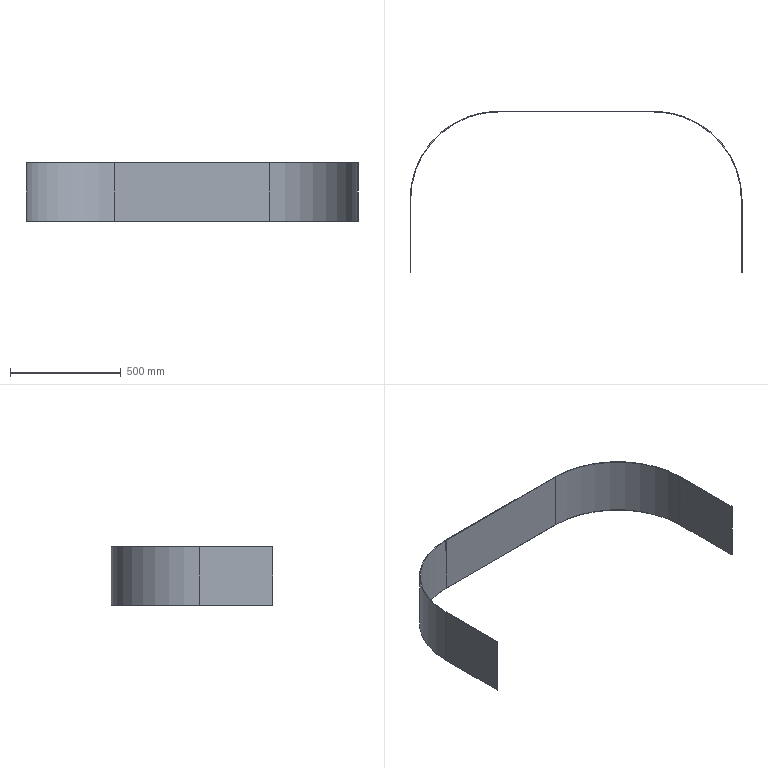Part | NX | features BREP 1 | 1 solid | 14 faces | box 1498 x 729 x 265 mm | volume 2073983 mm3 | plane 10 | cylinder 4 | commonest cylinder face diameters 792 x2 798 x2
STEP:
#1=CARTESIAN_POINT('',(746.,0.,-132.5));
#2=VERTEX_POINT('',#1);
#3=CARTESIAN_POINT('',(746.,-330.,-132.5));
#4=VERTEX_POINT('',#3);
#5=CARTESIAN_POINT('',(746.,0.,-132.5));
#6=DIRECTION('',(0.,-1.,0.));
#7=VECTOR('',#6,1000.);
#8=LINE('',#5,#7);
#9=EDGE_CURVE('',#2,#4,#8,.T.);
#10=ORIENTED_EDGE('',*,*,#9,.T.);
#11=CARTESIAN_POINT('',(746.,-330.,132.5));
#12=VERTEX_POINT('',#11);
#13=CARTESIAN_POINT('',(746.,-330.,132.5));
#14=DIRECTION('',(0.,0.,-1.));
#15=VECTOR('',#14,1000.);
#16=LINE('',#13,#15);
#17=EDGE_CURVE('',#12,#4,#16,.T.);
#18=ORIENTED_EDGE('',*,*,#17,.F.);
#19=CARTESIAN_POINT('',(746.,0.,132.5));
#20=VERTEX_POINT('',#19);
#21=CARTESIAN_POINT('',(746.,0.,132.5));
#22=DIRECTION('',(0.,-1.,0.));
#23=VECTOR('',#22,1000.);
#24=LINE('',#21,#23);
#25=EDGE_CURVE('',#20,#12,#24,.T.);
#26=ORIENTED_EDGE('',*,*,#25,.F.);
#27=CARTESIAN_POINT('',(746.,0.,132.5));
#28=DIRECTION('',(0.,0.,-1.));
#29=VECTOR('',#28,1000.);
#30=LINE('',#27,#29);
#31=EDGE_CURVE('',#20,#2,#30,.T.);
#32=ORIENTED_EDGE('',*,*,#31,.T.);
#33=EDGE_LOOP('',(#10,#18,#26,#32));
#34=FACE_BOUND('',#33,.T.);
#35=CARTESIAN_POINT('',(746.,0.,132.5));
#36=DIRECTION('',(1.,0.,0.));
#37=DIRECTION('',(0.,-1.,0.));
#38=AXIS2_PLACEMENT_3D('',#35,#36,#37);
#39=PLANE('',#38);
#40=ADVANCED_FACE('',(#34),#39,.F.);
#41=CARTESIAN_POINT('',(749.,-330.,-132.5));
#42=VERTEX_POINT('',#41);
#43=CARTESIAN_POINT('',(749.,-330.,-132.5));
#44=DIRECTION('',(-1.,0.,0.));
#45=VECTOR('',#44,1000.);
#46=LINE('',#43,#45);
#47=EDGE_CURVE('',#42,#4,#46,.T.);
#48=ORIENTED_EDGE('',*,*,#47,.F.);
#49=CARTESIAN_POINT('',(749.,-330.,132.5));
#50=VERTEX_POINT('',#49);
#51=CARTESIAN_POINT('',(749.,-330.,132.5));
#52=DIRECTION('',(0.,0.,-1.));
#53=VECTOR('',#52,1000.);
#54=LINE('',#51,#53);
#55=EDGE_CURVE('',#50,#42,#54,.T.);
#56=ORIENTED_EDGE('',*,*,#55,.F.);
#57=CARTESIAN_POINT('',(749.,-330.,132.5));
#58=DIRECTION('',(-1.,0.,0.));
#59=VECTOR('',#58,1000.);
#60=LINE('',#57,#59);
#61=EDGE_CURVE('',#50,#12,#60,.T.);
#62=ORIENTED_EDGE('',*,*,#61,.T.);
#63=ORIENTED_EDGE('',*,*,#17,.T.);
#64=EDGE_LOOP('',(#48,#56,#62,#63));
#65=FACE_BOUND('',#64,.T.);
#66=CARTESIAN_POINT('',(749.,-330.,132.5));
#67=DIRECTION('',(0.,-1.,0.));
#68=DIRECTION('',(0.,0.,1.));
#69=AXIS2_PLACEMENT_3D('',#66,#67,#68);
#70=PLANE('',#69);
#71=ADVANCED_FACE('',(#65),#70,.T.);
#72=CARTESIAN_POINT('',(749.,0.,-132.5));
#73=VERTEX_POINT('',#72);
#74=CARTESIAN_POINT('',(749.,0.,-132.5));
#75=DIRECTION('',(0.,-1.,0.));
#76=VECTOR('',#75,1000.);
#77=LINE('',#74,#76);
#78=EDGE_CURVE('',#73,#42,#77,.T.);
#79=ORIENTED_EDGE('',*,*,#78,.F.);
#80=CARTESIAN_POINT('',(749.,0.,132.5));
#81=VERTEX_POINT('',#80);
#82=CARTESIAN_POINT('',(749.,0.,132.5));
#83=DIRECTION('',(0.,0.,-1.));
#84=VECTOR('',#83,1000.);
#85=LINE('',#82,#84);
#86=EDGE_CURVE('',#81,#73,#85,.T.);
#87=ORIENTED_EDGE('',*,*,#86,.F.);
#88=CARTESIAN_POINT('',(749.,0.,132.5));
#89=DIRECTION('',(0.,-1.,0.));
#90=VECTOR('',#89,1000.);
#91=LINE('',#88,#90);
#92=EDGE_CURVE('',#81,#50,#91,.T.);
#93=ORIENTED_EDGE('',*,*,#92,.T.);
#94=ORIENTED_EDGE('',*,*,#55,.T.);
#95=EDGE_LOOP('',(#79,#87,#93,#94));
#96=FACE_BOUND('',#95,.T.);
#97=CARTESIAN_POINT('',(749.,0.,132.5));
#98=DIRECTION('',(1.,0.,0.));
#99=DIRECTION('',(0.,-1.,0.));
#100=AXIS2_PLACEMENT_3D('',#97,#98,#99);
#101=PLANE('',#100);
#102=ADVANCED_FACE('',(#96),#101,.T.);
#103=CARTESIAN_POINT('',(350.,399.,-132.5));
#104=VERTEX_POINT('',#103);
#105=CARTESIAN_POINT('',(350.,0.,-132.5));
#106=DIRECTION('',(0.,0.,-1.));
#107=DIRECTION('',(1.,0.,0.));
#108=AXIS2_PLACEMENT_3D('',#105,#106,#107);
#109=CIRCLE('',#108,399.);
#110=EDGE_CURVE('',#104,#73,#109,.T.);
#111=ORIENTED_EDGE('',*,*,#110,.F.);
#112=CARTESIAN_POINT('',(350.,399.,132.5));
#113=VERTEX_POINT('',#112);
#114=CARTESIAN_POINT('',(350.,399.,132.5));
#115=DIRECTION('',(0.,0.,-1.));
#116=VECTOR('',#115,1000.);
#117=LINE('',#114,#116);
#118=EDGE_CURVE('',#113,#104,#117,.T.);
#119=ORIENTED_EDGE('',*,*,#118,.F.);
#120=CARTESIAN_POINT('',(350.,0.,132.5));
#121=DIRECTION('',(0.,0.,-1.));
#122=DIRECTION('',(1.,0.,0.));
#123=AXIS2_PLACEMENT_3D('',#120,#121,#122);
#124=CIRCLE('',#123,399.);
#125=EDGE_CURVE('',#113,#81,#124,.T.);
#126=ORIENTED_EDGE('',*,*,#125,.T.);
#127=ORIENTED_EDGE('',*,*,#86,.T.);
#128=EDGE_LOOP('',(#111,#119,#126,#127));
#129=FACE_BOUND('',#128,.T.);
#130=CARTESIAN_POINT('',(350.,0.,132.5));
#131=DIRECTION('',(0.,0.,-1.));
#132=DIRECTION('',(1.,0.,0.));
#133=AXIS2_PLACEMENT_3D('',#130,#131,#132);
#134=CYLINDRICAL_SURFACE('',#133,399.);
#135=ADVANCED_FACE('',(#129),#134,.T.);
#136=CARTESIAN_POINT('',(-350.,399.,-132.5));
#137=VERTEX_POINT('',#136);
#138=CARTESIAN_POINT('',(-350.,399.,-132.5));
#139=DIRECTION('',(1.,0.,0.));
#140=VECTOR('',#139,1000.);
#141=LINE('',#138,#140);
#142=EDGE_CURVE('',#137,#104,#141,.T.);
#143=ORIENTED_EDGE('',*,*,#142,.F.);
#144=CARTESIAN_POINT('',(-350.,399.,132.5));
#145=VERTEX_POINT('',#144);
#146=CARTESIAN_POINT('',(-350.,399.,132.5));
#147=DIRECTION('',(0.,0.,-1.));
#148=VECTOR('',#147,1000.);
#149=LINE('',#146,#148);
#150=EDGE_CURVE('',#145,#137,#149,.T.);
#151=ORIENTED_EDGE('',*,*,#150,.F.);
#152=CARTESIAN_POINT('',(-350.,399.,132.5));
#153=DIRECTION('',(1.,0.,0.));
#154=VECTOR('',#153,1000.);
#155=LINE('',#152,#154);
#156=EDGE_CURVE('',#145,#113,#155,.T.);
#157=ORIENTED_EDGE('',*,*,#156,.T.);
#158=ORIENTED_EDGE('',*,*,#118,.T.);
#159=EDGE_LOOP('',(#143,#151,#157,#158));
#160=FACE_BOUND('',#159,.T.);
#161=CARTESIAN_POINT('',(-350.,399.,132.5));
#162=DIRECTION('',(0.,1.,0.));
#163=DIRECTION('',(1.,0.,0.));
#164=AXIS2_PLACEMENT_3D('',#161,#162,#163);
#165=PLANE('',#164);
#166=ADVANCED_FACE('',(#160),#165,.T.);
#167=CARTESIAN_POINT('',(-749.,0.,-132.5));
#168=VERTEX_POINT('',#167);
#169=CARTESIAN_POINT('',(-350.,0.,-132.5));
#170=DIRECTION('',(0.,0.,-1.));
#171=DIRECTION('',(1.,0.,0.));
#172=AXIS2_PLACEMENT_3D('',#169,#170,#171);
#173=CIRCLE('',#172,399.);
#174=EDGE_CURVE('',#168,#137,#173,.T.);
#175=ORIENTED_EDGE('',*,*,#174,.F.);
#176=CARTESIAN_POINT('',(-749.,0.,132.5));
#177=VERTEX_POINT('',#176);
#178=CARTESIAN_POINT('',(-749.,0.,132.5));
#179=DIRECTION('',(0.,0.,-1.));
#180=VECTOR('',#179,1000.);
#181=LINE('',#178,#180);
#182=EDGE_CURVE('',#177,#168,#181,.T.);
#183=ORIENTED_EDGE('',*,*,#182,.F.);
#184=CARTESIAN_POINT('',(-350.,0.,132.5));
#185=DIRECTION('',(0.,0.,-1.));
#186=DIRECTION('',(1.,0.,0.));
#187=AXIS2_PLACEMENT_3D('',#184,#185,#186);
#188=CIRCLE('',#187,399.);
#189=EDGE_CURVE('',#177,#145,#188,.T.);
#190=ORIENTED_EDGE('',*,*,#189,.T.);
#191=ORIENTED_EDGE('',*,*,#150,.T.);
#192=EDGE_LOOP('',(#175,#183,#190,#191));
#193=FACE_BOUND('',#192,.T.);
#194=CARTESIAN_POINT('',(-350.,0.,132.5));
#195=DIRECTION('',(0.,0.,-1.));
#196=DIRECTION('',(1.,0.,0.));
#197=AXIS2_PLACEMENT_3D('',#194,#195,#196);
#198=CYLINDRICAL_SURFACE('',#197,399.);
#199=ADVANCED_FACE('',(#193),#198,.T.);
#200=CARTESIAN_POINT('',(-749.,-330.,-132.5));
#201=VERTEX_POINT('',#200);
#202=CARTESIAN_POINT('',(-749.,0.,-132.5));
#203=DIRECTION('',(0.,1.,0.));
#204=VECTOR('',#203,1000.);
#205=LINE('',#202,#204);
#206=EDGE_CURVE('',#201,#168,#205,.T.);
#207=ORIENTED_EDGE('',*,*,#206,.F.);
#208=CARTESIAN_POINT('',(-749.,-330.,132.5));
#209=VERTEX_POINT('',#208);
#210=CARTESIAN_POINT('',(-749.,-330.,132.5));
#211=DIRECTION('',(0.,0.,-1.));
#212=VECTOR('',#211,1000.);
#213=LINE('',#210,#212);
#214=EDGE_CURVE('',#209,#201,#213,.T.);
#215=ORIENTED_EDGE('',*,*,#214,.F.);
#216=CARTESIAN_POINT('',(-749.,0.,132.5));
#217=DIRECTION('',(0.,1.,0.));
#218=VECTOR('',#217,1000.);
#219=LINE('',#216,#218);
#220=EDGE_CURVE('',#209,#177,#219,.T.);
#221=ORIENTED_EDGE('',*,*,#220,.T.);
#222=ORIENTED_EDGE('',*,*,#182,.T.);
#223=EDGE_LOOP('',(#207,#215,#221,#222));
#224=FACE_BOUND('',#223,.T.);
#225=CARTESIAN_POINT('',(-749.,0.,132.5));
#226=DIRECTION('',(-1.,0.,0.));
#227=DIRECTION('',(0.,1.,0.));
#228=AXIS2_PLACEMENT_3D('',#225,#226,#227);
#229=PLANE('',#228);
#230=ADVANCED_FACE('',(#224),#229,.T.);
#231=CARTESIAN_POINT('',(-746.,-330.,-132.5));
#232=VERTEX_POINT('',#231);
#233=CARTESIAN_POINT('',(-746.,-330.,-132.5));
#234=DIRECTION('',(-1.,0.,0.));
#235=VECTOR('',#234,1000.);
#236=LINE('',#233,#235);
#237=EDGE_CURVE('',#232,#201,#236,.T.);
#238=ORIENTED_EDGE('',*,*,#237,.F.);
#239=CARTESIAN_POINT('',(-746.,-330.,132.5));
#240=VERTEX_POINT('',#239);
#241=CARTESIAN_POINT('',(-746.,-330.,132.5));
#242=DIRECTION('',(0.,0.,-1.));
#243=VECTOR('',#242,1000.);
#244=LINE('',#241,#243);
#245=EDGE_CURVE('',#240,#232,#244,.T.);
#246=ORIENTED_EDGE('',*,*,#245,.F.);
#247=CARTESIAN_POINT('',(-746.,-330.,132.5));
#248=DIRECTION('',(-1.,0.,0.));
#249=VECTOR('',#248,1000.);
#250=LINE('',#247,#249);
#251=EDGE_CURVE('',#240,#209,#250,.T.);
#252=ORIENTED_EDGE('',*,*,#251,.T.);
#253=ORIENTED_EDGE('',*,*,#214,.T.);
#254=EDGE_LOOP('',(#238,#246,#252,#253));
#255=FACE_BOUND('',#254,.T.);
#256=CARTESIAN_POINT('',(-746.,-330.,132.5));
#257=DIRECTION('',(0.,-1.,0.));
#258=DIRECTION('',(0.,0.,1.));
#259=AXIS2_PLACEMENT_3D('',#256,#257,#258);
#260=PLANE('',#259);
#261=ADVANCED_FACE('',(#255),#260,.T.);
#262=CARTESIAN_POINT('',(-746.,0.,-132.5));
#263=VERTEX_POINT('',#262);
#264=CARTESIAN_POINT('',(-746.,0.,-132.5));
#265=DIRECTION('',(0.,1.,0.));
#266=VECTOR('',#265,1000.);
#267=LINE('',#264,#266);
#268=EDGE_CURVE('',#232,#263,#267,.T.);
#269=ORIENTED_EDGE('',*,*,#268,.T.);
#270=CARTESIAN_POINT('',(-746.,0.,132.5));
#271=VERTEX_POINT('',#270);
#272=CARTESIAN_POINT('',(-746.,0.,132.5));
#273=DIRECTION('',(0.,0.,-1.));
#274=VECTOR('',#273,1000.);
#275=LINE('',#272,#274);
#276=EDGE_CURVE('',#271,#263,#275,.T.);
#277=ORIENTED_EDGE('',*,*,#276,.F.);
#278=CARTESIAN_POINT('',(-746.,0.,132.5));
#279=DIRECTION('',(0.,1.,0.));
#280=VECTOR('',#279,1000.);
#281=LINE('',#278,#280);
#282=EDGE_CURVE('',#240,#271,#281,.T.);
#283=ORIENTED_EDGE('',*,*,#282,.F.);
#284=ORIENTED_EDGE('',*,*,#245,.T.);
#285=EDGE_LOOP('',(#269,#277,#283,#284));
#286=FACE_BOUND('',#285,.T.);
#287=CARTESIAN_POINT('',(-746.,0.,132.5));
#288=DIRECTION('',(-1.,0.,0.));
#289=DIRECTION('',(0.,1.,0.));
#290=AXIS2_PLACEMENT_3D('',#287,#288,#289);
#291=PLANE('',#290);
#292=ADVANCED_FACE('',(#286),#291,.F.);
#293=CARTESIAN_POINT('',(-350.,396.,-132.5));
#294=VERTEX_POINT('',#293);
#295=CARTESIAN_POINT('',(-350.,0.,-132.5));
#296=DIRECTION('',(0.,0.,-1.));
#297=DIRECTION('',(1.,0.,0.));
#298=AXIS2_PLACEMENT_3D('',#295,#296,#297);
#299=CIRCLE('',#298,396.);
#300=EDGE_CURVE('',#263,#294,#299,.T.);
#301=ORIENTED_EDGE('',*,*,#300,.T.);
#302=CARTESIAN_POINT('',(-350.,396.,132.5));
#303=VERTEX_POINT('',#302);
#304=CARTESIAN_POINT('',(-350.,396.,132.5));
#305=DIRECTION('',(0.,0.,-1.));
#306=VECTOR('',#305,1000.);
#307=LINE('',#304,#306);
#308=EDGE_CURVE('',#303,#294,#307,.T.);
#309=ORIENTED_EDGE('',*,*,#308,.F.);
#310=CARTESIAN_POINT('',(-350.,0.,132.5));
#311=DIRECTION('',(0.,0.,-1.));
#312=DIRECTION('',(1.,0.,0.));
#313=AXIS2_PLACEMENT_3D('',#310,#311,#312);
#314=CIRCLE('',#313,396.);
#315=EDGE_CURVE('',#271,#303,#314,.T.);
#316=ORIENTED_EDGE('',*,*,#315,.F.);
#317=ORIENTED_EDGE('',*,*,#276,.T.);
#318=EDGE_LOOP('',(#301,#309,#316,#317));
#319=FACE_BOUND('',#318,.T.);
#320=CARTESIAN_POINT('',(-350.,0.,132.5));
#321=DIRECTION('',(0.,0.,-1.));
#322=DIRECTION('',(1.,0.,0.));
#323=AXIS2_PLACEMENT_3D('',#320,#321,#322);
#324=CYLINDRICAL_SURFACE('',#323,396.);
#325=ADVANCED_FACE('',(#319),#324,.F.);
#326=CARTESIAN_POINT('',(350.,396.,-132.5));
#327=VERTEX_POINT('',#326);
#328=CARTESIAN_POINT('',(-350.,396.,-132.5));
#329=DIRECTION('',(1.,0.,0.));
#330=VECTOR('',#329,1000.);
#331=LINE('',#328,#330);
#332=EDGE_CURVE('',#294,#327,#331,.T.);
#333=ORIENTED_EDGE('',*,*,#332,.T.);
#334=CARTESIAN_POINT('',(350.,396.,132.5));
#335=VERTEX_POINT('',#334);
#336=CARTESIAN_POINT('',(350.,396.,132.5));
#337=DIRECTION('',(0.,0.,-1.));
#338=VECTOR('',#337,1000.);
#339=LINE('',#336,#338);
#340=EDGE_CURVE('',#335,#327,#339,.T.);
#341=ORIENTED_EDGE('',*,*,#340,.F.);
#342=CARTESIAN_POINT('',(-350.,396.,132.5));
#343=DIRECTION('',(1.,0.,0.));
#344=VECTOR('',#343,1000.);
#345=LINE('',#342,#344);
#346=EDGE_CURVE('',#303,#335,#345,.T.);
#347=ORIENTED_EDGE('',*,*,#346,.F.);
#348=ORIENTED_EDGE('',*,*,#308,.T.);
#349=EDGE_LOOP('',(#333,#341,#347,#348));
#350=FACE_BOUND('',#349,.T.);
#351=CARTESIAN_POINT('',(-350.,396.,132.5));
#352=DIRECTION('',(0.,1.,0.));
#353=DIRECTION('',(1.,0.,0.));
#354=AXIS2_PLACEMENT_3D('',#351,#352,#353);
#355=PLANE('',#354);
#356=ADVANCED_FACE('',(#350),#355,.F.);
#357=CARTESIAN_POINT('',(350.,0.,-132.5));
#358=DIRECTION('',(0.,0.,-1.));
#359=DIRECTION('',(-1.,0.,0.));
#360=AXIS2_PLACEMENT_3D('',#357,#358,#359);
#361=CIRCLE('',#360,396.);
#362=EDGE_CURVE('',#327,#2,#361,.T.);
#363=ORIENTED_EDGE('',*,*,#362,.T.);
#364=ORIENTED_EDGE('',*,*,#31,.F.);
#365=CARTESIAN_POINT('',(350.,0.,132.5));
#366=DIRECTION('',(0.,0.,-1.));
#367=DIRECTION('',(-1.,0.,0.));
#368=AXIS2_PLACEMENT_3D('',#365,#366,#367);
#369=CIRCLE('',#368,396.);
#370=EDGE_CURVE('',#335,#20,#369,.T.);
#371=ORIENTED_EDGE('',*,*,#370,.F.);
#372=ORIENTED_EDGE('',*,*,#340,.T.);
#373=EDGE_LOOP('',(#363,#364,#371,#372));
#374=FACE_BOUND('',#373,.T.);
#375=CARTESIAN_POINT('',(350.,0.,132.5));
#376=DIRECTION('',(0.,0.,-1.));
#377=DIRECTION('',(1.,0.,0.));
#378=AXIS2_PLACEMENT_3D('',#375,#376,#377);
#379=CYLINDRICAL_SURFACE('',#378,396.);
#380=ADVANCED_FACE('',(#374),#379,.F.);
#381=ORIENTED_EDGE('',*,*,#25,.T.);
#382=ORIENTED_EDGE('',*,*,#61,.F.);
#383=ORIENTED_EDGE('',*,*,#92,.F.);
#384=ORIENTED_EDGE('',*,*,#125,.F.);
#385=ORIENTED_EDGE('',*,*,#156,.F.);
#386=ORIENTED_EDGE('',*,*,#189,.F.);
#387=ORIENTED_EDGE('',*,*,#220,.F.);
#388=ORIENTED_EDGE('',*,*,#251,.F.);
#389=ORIENTED_EDGE('',*,*,#282,.T.);
#390=ORIENTED_EDGE('',*,*,#315,.T.);
#391=ORIENTED_EDGE('',*,*,#346,.T.);
#392=ORIENTED_EDGE('',*,*,#370,.T.);
#393=EDGE_LOOP('',(#381,#382,#383,#384,#385,#386,#387,#388,#389,#390,#391,#392));
#394=FACE_BOUND('',#393,.T.);
#395=CARTESIAN_POINT('',(350.,0.,132.5));
#396=DIRECTION('',(0.,0.,1.));
#397=DIRECTION('',(-1.,0.,0.));
#398=AXIS2_PLACEMENT_3D('',#395,#396,#397);
#399=PLANE('',#398);
#400=ADVANCED_FACE('',(#394),#399,.T.);
#401=ORIENTED_EDGE('',*,*,#9,.F.);
#402=ORIENTED_EDGE('',*,*,#362,.F.);
#403=ORIENTED_EDGE('',*,*,#332,.F.);
#404=ORIENTED_EDGE('',*,*,#300,.F.);
#405=ORIENTED_EDGE('',*,*,#268,.F.);
#406=ORIENTED_EDGE('',*,*,#237,.T.);
#407=ORIENTED_EDGE('',*,*,#206,.T.);
#408=ORIENTED_EDGE('',*,*,#174,.T.);
#409=ORIENTED_EDGE('',*,*,#142,.T.);
#410=ORIENTED_EDGE('',*,*,#110,.T.);
#411=ORIENTED_EDGE('',*,*,#78,.T.);
#412=ORIENTED_EDGE('',*,*,#47,.T.);
#413=EDGE_LOOP('',(#401,#402,#403,#404,#405,#406,#407,#408,#409,#410,#411,#412));
#414=FACE_BOUND('',#413,.T.);
#415=CARTESIAN_POINT('',(350.,0.,-132.5));
#416=DIRECTION('',(0.,0.,1.));
#417=DIRECTION('',(-1.,0.,0.));
#418=AXIS2_PLACEMENT_3D('',#415,#416,#417);
#419=PLANE('',#418);
#420=ADVANCED_FACE('',(#414),#419,.F.);
#421=CLOSED_SHELL('',(#40,#71,#102,#135,#166,#199,#230,#261,#292,#325,#356,#380,#400,#420));
#422=MANIFOLD_SOLID_BREP('',#421);
#423=(LENGTH_UNIT()NAMED_UNIT(*)SI_UNIT(.MILLI.,.METRE.));
#424=UNCERTAINTY_MEASURE_WITH_UNIT(LENGTH_MEASURE(0.00001),#423,'','');
#425=(NAMED_UNIT(*)PLANE_ANGLE_UNIT()SI_UNIT($,.RADIAN.));
#426=(NAMED_UNIT(*)SI_UNIT($,.STERADIAN.)SOLID_ANGLE_UNIT());
#427=(GEOMETRIC_REPRESENTATION_CONTEXT(3)GLOBAL_UNCERTAINTY_ASSIGNED_CONTEXT((#424))GLOBAL_UNIT_ASSIGNED_CONTEXT((#423,#425,#426))REPRESENTATION_CONTEXT('',''));
#428=ADVANCED_BREP_SHAPE_REPRESENTATION('',(#422),#427);